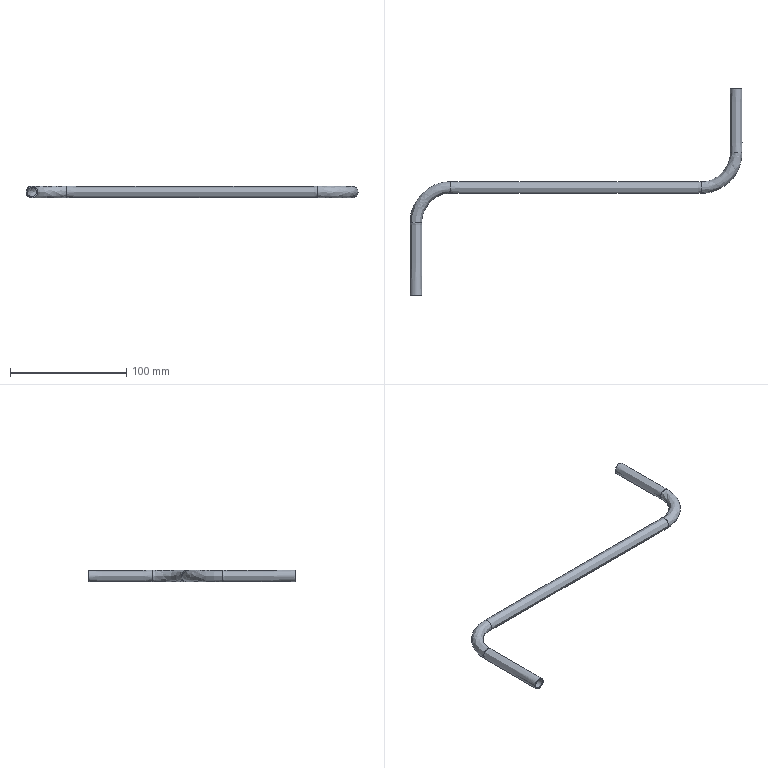Part | NX | features solid 2 | 1 solid | 12 faces | box 285.01 x 177.608 x 10 mm | volume 12034 mm3 | spline 11 | plane 1